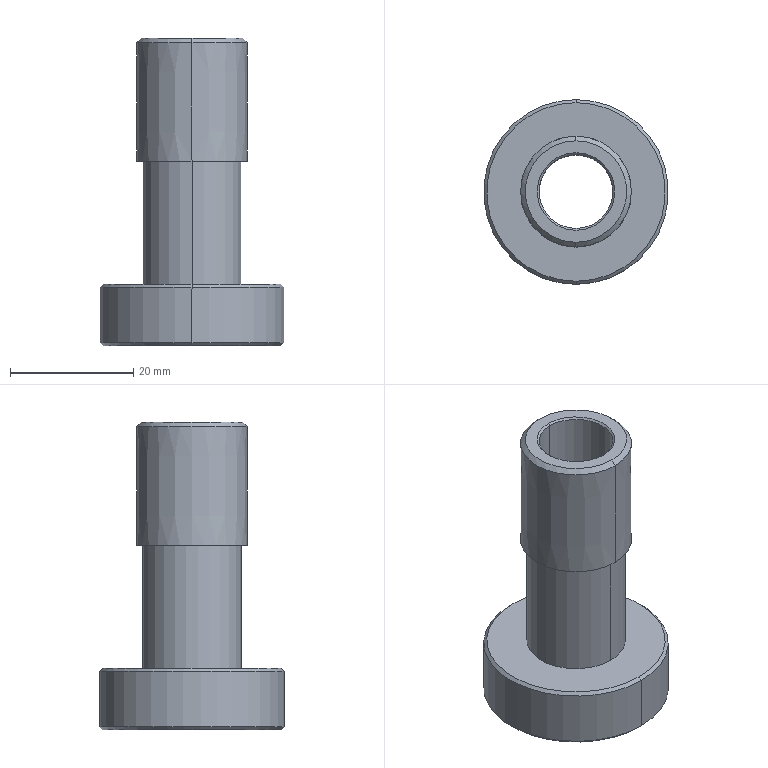Part | SolidWorks | features BaseBody 1 | 1 solid | 32 faces | box 30 x 30 x 50 mm | volume 10165 mm3 | cone 16 | cylinder 10 | plane 6 | commonest cylinder face diameters 5 x4 12 x2 16 x2 30 x2
STEP:
#1=CARTESIAN_POINT('',(590.535,44.349,-74.93));
#2=VERTEX_POINT('',#1);
#3=CARTESIAN_POINT('',(590.535,32.349,-74.93));
#4=VERTEX_POINT('',#3);
#5=CARTESIAN_POINT('',(590.535,38.349,-74.93));
#6=DIRECTION('',(0.,0.,1.));
#7=DIRECTION('',(0.,-1.,0.));
#8=AXIS2_PLACEMENT_3D('',#5,#6,#7);
#9=CIRCLE('',#8,6.);
#10=EDGE_CURVE('',#2,#4,#9,.T.);
#11=ORIENTED_EDGE('',*,*,#10,.F.);
#12=CARTESIAN_POINT('',(590.535,44.349,-25.53));
#13=VERTEX_POINT('',#12);
#14=CARTESIAN_POINT('',(590.535,44.349,-75.23));
#15=DIRECTION('',(0.,0.,1.));
#16=VECTOR('',#15,1000.);
#17=LINE('',#14,#16);
#18=EDGE_CURVE('',#2,#13,#17,.T.);
#19=ORIENTED_EDGE('',*,*,#18,.T.);
#20=CARTESIAN_POINT('',(590.535,32.349,-25.53));
#21=VERTEX_POINT('',#20);
#22=CARTESIAN_POINT('',(590.535,38.349,-25.53));
#23=DIRECTION('',(0.,0.,-1.));
#24=DIRECTION('',(0.,-1.,0.));
#25=AXIS2_PLACEMENT_3D('',#22,#23,#24);
#26=CIRCLE('',#25,6.);
#27=EDGE_CURVE('',#21,#13,#26,.T.);
#28=ORIENTED_EDGE('',*,*,#27,.F.);
#29=CARTESIAN_POINT('',(590.535,32.349,-75.23));
#30=DIRECTION('',(0.,0.,1.));
#31=VECTOR('',#30,1000.);
#32=LINE('',#29,#31);
#33=EDGE_CURVE('',#4,#21,#32,.T.);
#34=ORIENTED_EDGE('',*,*,#33,.F.);
#35=EDGE_LOOP('',(#11,#19,#28,#34));
#36=FACE_OUTER_BOUND('',#35,.T.);
#37=CARTESIAN_POINT('',(590.535,38.349,-75.23));
#38=DIRECTION('',(0.,0.,1.));
#39=DIRECTION('',(0.,-1.,0.));
#40=AXIS2_PLACEMENT_3D('',#37,#38,#39);
#41=CYLINDRICAL_SURFACE('',#40,6.);
#42=ADVANCED_FACE('',(#36),#41,.F.);
#43=ORIENTED_EDGE('',*,*,#10,.T.);
#44=CARTESIAN_POINT('',(590.535,32.049,-75.23));
#45=VERTEX_POINT('',#44);
#46=CARTESIAN_POINT('',(590.535,32.049,-75.23));
#47=DIRECTION('',(0.,-0.7071,-0.7071));
#48=VECTOR('',#47,1000.);
#49=LINE('',#46,#48);
#50=EDGE_CURVE('',#4,#45,#49,.T.);
#51=ORIENTED_EDGE('',*,*,#50,.T.);
#52=CARTESIAN_POINT('',(590.535,44.649,-75.23));
#53=VERTEX_POINT('',#52);
#54=CARTESIAN_POINT('',(590.535,38.349,-75.23));
#55=DIRECTION('',(0.,0.,1.));
#56=DIRECTION('',(0.,1.,0.));
#57=AXIS2_PLACEMENT_3D('',#54,#55,#56);
#58=CIRCLE('',#57,6.3);
#59=EDGE_CURVE('',#53,#45,#58,.T.);
#60=ORIENTED_EDGE('',*,*,#59,.F.);
#61=CARTESIAN_POINT('',(590.535,44.649,-75.23));
#62=DIRECTION('',(0.,0.7071,-0.7071));
#63=VECTOR('',#62,1000.);
#64=LINE('',#61,#63);
#65=EDGE_CURVE('',#2,#53,#64,.T.);
#66=ORIENTED_EDGE('',*,*,#65,.F.);
#67=EDGE_LOOP('',(#43,#51,#60,#66));
#68=FACE_OUTER_BOUND('',#67,.T.);
#69=CARTESIAN_POINT('',(590.535,38.349,-75.23));
#70=DIRECTION('',(0.,0.,-1.));
#71=DIRECTION('',(0.,1.,0.));
#72=AXIS2_PLACEMENT_3D('',#69,#70,#71);
#73=CONICAL_SURFACE('',#72,6.3,0.7854);
#74=ADVANCED_FACE('',(#68),#73,.F.);
#75=ORIENTED_EDGE('',*,*,#27,.T.);
#76=CARTESIAN_POINT('',(590.535,44.649,-25.23));
#77=VERTEX_POINT('',#76);
#78=CARTESIAN_POINT('',(590.535,44.649,-25.23));
#79=DIRECTION('',(0.,0.7071,0.7071));
#80=VECTOR('',#79,1000.);
#81=LINE('',#78,#80);
#82=EDGE_CURVE('',#13,#77,#81,.T.);
#83=ORIENTED_EDGE('',*,*,#82,.T.);
#84=CARTESIAN_POINT('',(590.535,32.049,-25.23));
#85=VERTEX_POINT('',#84);
#86=CARTESIAN_POINT('',(590.535,38.349,-25.23));
#87=DIRECTION('',(0.,0.,-1.));
#88=DIRECTION('',(0.,-1.,0.));
#89=AXIS2_PLACEMENT_3D('',#86,#87,#88);
#90=CIRCLE('',#89,6.3);
#91=EDGE_CURVE('',#85,#77,#90,.T.);
#92=ORIENTED_EDGE('',*,*,#91,.F.);
#93=CARTESIAN_POINT('',(590.535,32.049,-25.23));
#94=DIRECTION('',(0.,-0.7071,0.7071));
#95=VECTOR('',#94,1000.);
#96=LINE('',#93,#95);
#97=EDGE_CURVE('',#21,#85,#96,.T.);
#98=ORIENTED_EDGE('',*,*,#97,.F.);
#99=EDGE_LOOP('',(#75,#83,#92,#98));
#100=FACE_OUTER_BOUND('',#99,.T.);
#101=CARTESIAN_POINT('',(590.535,38.349,-25.23));
#102=DIRECTION('',(0.,0.,1.));
#103=DIRECTION('',(0.,-1.,0.));
#104=AXIS2_PLACEMENT_3D('',#101,#102,#103);
#105=CONICAL_SURFACE('',#104,6.3,0.7854);
#106=ADVANCED_FACE('',(#100),#105,.F.);
#107=CARTESIAN_POINT('',(596.909,43.555,-74.93));
#108=VERTEX_POINT('',#107);
#109=CARTESIAN_POINT('',(596.909,48.555,-74.93));
#110=VERTEX_POINT('',#109);
#111=CARTESIAN_POINT('',(596.909,46.055,-74.93));
#112=DIRECTION('',(0.,0.,-1.));
#113=DIRECTION('',(0.6374,0.7706,0.));
#114=AXIS2_PLACEMENT_3D('',#111,#112,#113);
#115=CIRCLE('',#114,2.5);
#116=EDGE_CURVE('',#108,#110,#115,.T.);
#117=ORIENTED_EDGE('',*,*,#116,.F.);
#118=CARTESIAN_POINT('',(596.909,43.255,-75.23));
#119=VERTEX_POINT('',#118);
#120=CARTESIAN_POINT('',(596.909,43.255,-75.23));
#121=DIRECTION('',(0.,-0.7071,-0.7071));
#122=VECTOR('',#121,1000.);
#123=LINE('',#120,#122);
#124=EDGE_CURVE('',#108,#119,#123,.T.);
#125=ORIENTED_EDGE('',*,*,#124,.T.);
#126=CARTESIAN_POINT('',(596.909,48.855,-75.23));
#127=VERTEX_POINT('',#126);
#128=CARTESIAN_POINT('',(596.909,46.055,-75.23));
#129=DIRECTION('',(0.,0.,-1.));
#130=DIRECTION('',(0.,1.,0.));
#131=AXIS2_PLACEMENT_3D('',#128,#129,#130);
#132=CIRCLE('',#131,2.8);
#133=EDGE_CURVE('',#119,#127,#132,.T.);
#134=ORIENTED_EDGE('',*,*,#133,.T.);
#135=CARTESIAN_POINT('',(596.909,48.855,-75.23));
#136=DIRECTION('',(0.,0.7071,-0.7071));
#137=VECTOR('',#136,1000.);
#138=LINE('',#135,#137);
#139=EDGE_CURVE('',#110,#127,#138,.T.);
#140=ORIENTED_EDGE('',*,*,#139,.F.);
#141=EDGE_LOOP('',(#117,#125,#134,#140));
#142=FACE_OUTER_BOUND('',#141,.T.);
#143=CARTESIAN_POINT('',(596.909,46.055,-75.23));
#144=DIRECTION('',(0.,0.,-1.));
#145=DIRECTION('',(0.,1.,0.));
#146=AXIS2_PLACEMENT_3D('',#143,#144,#145);
#147=CONICAL_SURFACE('',#146,2.8,0.7854);
#148=ADVANCED_FACE('',(#142),#147,.F.);
#149=CARTESIAN_POINT('',(590.535,23.849,-75.23));
#150=VERTEX_POINT('',#149);
#151=CARTESIAN_POINT('',(590.535,52.849,-75.23));
#152=VERTEX_POINT('',#151);
#153=CARTESIAN_POINT('',(590.535,38.349,-75.23));
#154=DIRECTION('',(0.,0.,1.));
#155=DIRECTION('',(0.,-1.,0.));
#156=AXIS2_PLACEMENT_3D('',#153,#154,#155);
#157=CIRCLE('',#156,14.5);
#158=EDGE_CURVE('',#150,#152,#157,.T.);
#159=ORIENTED_EDGE('',*,*,#158,.T.);
#160=CARTESIAN_POINT('',(590.535,53.349,-74.73));
#161=VERTEX_POINT('',#160);
#162=CARTESIAN_POINT('',(590.535,53.349,-74.73));
#163=DIRECTION('',(0.,0.7071,0.7071));
#164=VECTOR('',#163,1000.);
#165=LINE('',#162,#164);
#166=EDGE_CURVE('',#152,#161,#165,.T.);
#167=ORIENTED_EDGE('',*,*,#166,.T.);
#168=CARTESIAN_POINT('',(590.535,23.349,-74.73));
#169=VERTEX_POINT('',#168);
#170=CARTESIAN_POINT('',(590.535,38.349,-74.73));
#171=DIRECTION('',(0.,0.,-1.));
#172=DIRECTION('',(0.6374,0.7706,0.));
#173=AXIS2_PLACEMENT_3D('',#170,#171,#172);
#174=CIRCLE('',#173,15.);
#175=EDGE_CURVE('',#161,#169,#174,.T.);
#176=ORIENTED_EDGE('',*,*,#175,.T.);
#177=CARTESIAN_POINT('',(590.535,23.349,-74.73));
#178=DIRECTION('',(0.,-0.7071,0.7071));
#179=VECTOR('',#178,1000.);
#180=LINE('',#177,#179);
#181=EDGE_CURVE('',#150,#169,#180,.T.);
#182=ORIENTED_EDGE('',*,*,#181,.F.);
#183=EDGE_LOOP('',(#159,#167,#176,#182));
#184=FACE_OUTER_BOUND('',#183,.T.);
#185=CARTESIAN_POINT('',(590.535,38.349,-74.73));
#186=DIRECTION('',(0.,0.,1.));
#187=DIRECTION('',(0.,-1.,0.));
#188=AXIS2_PLACEMENT_3D('',#185,#186,#187);
#189=CONICAL_SURFACE('',#188,15.,0.7854);
#190=ADVANCED_FACE('',(#184),#189,.T.);
#191=CARTESIAN_POINT('',(584.162,28.144,-74.93));
#192=VERTEX_POINT('',#191);
#193=CARTESIAN_POINT('',(584.162,33.144,-74.93));
#194=VERTEX_POINT('',#193);
#195=CARTESIAN_POINT('',(584.162,30.644,-74.93));
#196=DIRECTION('',(0.,0.,-1.));
#197=DIRECTION('',(0.6374,0.7706,0.));
#198=AXIS2_PLACEMENT_3D('',#195,#196,#197);
#199=CIRCLE('',#198,2.5);
#200=EDGE_CURVE('',#192,#194,#199,.T.);
#201=ORIENTED_EDGE('',*,*,#200,.F.);
#202=CARTESIAN_POINT('',(584.162,27.844,-75.23));
#203=VERTEX_POINT('',#202);
#204=CARTESIAN_POINT('',(584.162,27.844,-75.23));
#205=DIRECTION('',(0.,-0.7071,-0.7071));
#206=VECTOR('',#205,1000.);
#207=LINE('',#204,#206);
#208=EDGE_CURVE('',#192,#203,#207,.T.);
#209=ORIENTED_EDGE('',*,*,#208,.T.);
#210=CARTESIAN_POINT('',(584.162,33.444,-75.23));
#211=VERTEX_POINT('',#210);
#212=CARTESIAN_POINT('',(584.162,30.644,-75.23));
#213=DIRECTION('',(0.,0.,-1.));
#214=DIRECTION('',(0.,1.,0.));
#215=AXIS2_PLACEMENT_3D('',#212,#213,#214);
#216=CIRCLE('',#215,2.8);
#217=EDGE_CURVE('',#203,#211,#216,.T.);
#218=ORIENTED_EDGE('',*,*,#217,.T.);
#219=CARTESIAN_POINT('',(584.162,33.444,-75.23));
#220=DIRECTION('',(0.,0.7071,-0.7071));
#221=VECTOR('',#220,1000.);
#222=LINE('',#219,#221);
#223=EDGE_CURVE('',#194,#211,#222,.T.);
#224=ORIENTED_EDGE('',*,*,#223,.F.);
#225=EDGE_LOOP('',(#201,#209,#218,#224));
#226=FACE_OUTER_BOUND('',#225,.T.);
#227=CARTESIAN_POINT('',(584.162,30.644,-75.23));
#228=DIRECTION('',(0.,0.,-1.));
#229=DIRECTION('',(0.,1.,0.));
#230=AXIS2_PLACEMENT_3D('',#227,#228,#229);
#231=CONICAL_SURFACE('',#230,2.8,0.7854);
#232=ADVANCED_FACE('',(#226),#231,.F.);
#233=CARTESIAN_POINT('',(590.535,30.103,-25.23));
#234=VERTEX_POINT('',#233);
#235=CARTESIAN_POINT('',(590.535,46.596,-25.23));
#236=VERTEX_POINT('',#235);
#237=CARTESIAN_POINT('',(590.535,38.349,-25.23));
#238=DIRECTION('',(0.,0.,1.));
#239=DIRECTION('',(0.,1.,0.));
#240=AXIS2_PLACEMENT_3D('',#237,#238,#239);
#241=CIRCLE('',#240,8.247);
#242=EDGE_CURVE('',#234,#236,#241,.T.);
#243=ORIENTED_EDGE('',*,*,#242,.F.);
#244=CARTESIAN_POINT('',(590.535,29.353,-25.98));
#245=VERTEX_POINT('',#244);
#246=CARTESIAN_POINT('',(590.535,29.353,-25.98));
#247=DIRECTION('',(0.,-0.7072,-0.707));
#248=VECTOR('',#247,1000.);
#249=LINE('',#246,#248);
#250=EDGE_CURVE('',#234,#245,#249,.T.);
#251=ORIENTED_EDGE('',*,*,#250,.T.);
#252=CARTESIAN_POINT('',(590.535,47.346,-25.98));
#253=VERTEX_POINT('',#252);
#254=CARTESIAN_POINT('',(590.535,38.349,-25.98));
#255=DIRECTION('',(0.,0.,1.));
#256=DIRECTION('',(0.6374,0.7706,0.));
#257=AXIS2_PLACEMENT_3D('',#254,#255,#256);
#258=CIRCLE('',#257,8.997);
#259=EDGE_CURVE('',#245,#253,#258,.T.);
#260=ORIENTED_EDGE('',*,*,#259,.T.);
#261=CARTESIAN_POINT('',(590.535,47.346,-25.98));
#262=DIRECTION('',(0.,0.7072,-0.707));
#263=VECTOR('',#262,1000.);
#264=LINE('',#261,#263);
#265=EDGE_CURVE('',#236,#253,#264,.T.);
#266=ORIENTED_EDGE('',*,*,#265,.F.);
#267=EDGE_LOOP('',(#243,#251,#260,#266));
#268=FACE_OUTER_BOUND('',#267,.T.);
#269=CARTESIAN_POINT('',(590.535,38.349,-25.98));
#270=DIRECTION('',(0.,0.,-1.));
#271=DIRECTION('',(0.,1.,0.));
#272=AXIS2_PLACEMENT_3D('',#269,#270,#271);
#273=CONICAL_SURFACE('',#272,8.997,0.7855);
#274=ADVANCED_FACE('',(#268),#273,.T.);
#275=ORIENTED_EDGE('',*,*,#116,.T.);
#276=CARTESIAN_POINT('',(596.909,48.555,-67.23));
#277=VERTEX_POINT('',#276);
#278=CARTESIAN_POINT('',(596.909,48.555,-75.23));
#279=DIRECTION('',(0.,0.,1.));
#280=VECTOR('',#279,1000.);
#281=LINE('',#278,#280);
#282=EDGE_CURVE('',#110,#277,#281,.T.);
#283=ORIENTED_EDGE('',*,*,#282,.T.);
#284=CARTESIAN_POINT('',(596.909,43.555,-67.23));
#285=VERTEX_POINT('',#284);
#286=CARTESIAN_POINT('',(596.909,46.055,-67.23));
#287=DIRECTION('',(0.,0.,-1.));
#288=DIRECTION('',(0.,-1.,0.));
#289=AXIS2_PLACEMENT_3D('',#286,#287,#288);
#290=CIRCLE('',#289,2.5);
#291=EDGE_CURVE('',#285,#277,#290,.T.);
#292=ORIENTED_EDGE('',*,*,#291,.F.);
#293=CARTESIAN_POINT('',(596.909,43.555,-75.23));
#294=DIRECTION('',(0.,0.,1.));
#295=VECTOR('',#294,1000.);
#296=LINE('',#293,#295);
#297=EDGE_CURVE('',#108,#285,#296,.T.);
#298=ORIENTED_EDGE('',*,*,#297,.F.);
#299=EDGE_LOOP('',(#275,#283,#292,#298));
#300=FACE_OUTER_BOUND('',#299,.T.);
#301=CARTESIAN_POINT('',(596.909,46.055,-75.23));
#302=DIRECTION('',(0.,0.,1.));
#303=DIRECTION('',(0.,-1.,0.));
#304=AXIS2_PLACEMENT_3D('',#301,#302,#303);
#305=CYLINDRICAL_SURFACE('',#304,2.5);
#306=ADVANCED_FACE('',(#300),#305,.F.);
#307=ORIENTED_EDGE('',*,*,#175,.F.);
#308=CARTESIAN_POINT('',(590.535,53.349,-65.73));
#309=VERTEX_POINT('',#308);
#310=CARTESIAN_POINT('',(590.535,53.349,-75.23));
#311=DIRECTION('',(0.,0.,1.));
#312=VECTOR('',#311,1000.);
#313=LINE('',#310,#312);
#314=EDGE_CURVE('',#161,#309,#313,.T.);
#315=ORIENTED_EDGE('',*,*,#314,.T.);
#316=CARTESIAN_POINT('',(590.535,23.349,-65.73));
#317=VERTEX_POINT('',#316);
#318=CARTESIAN_POINT('',(590.535,38.349,-65.73));
#319=DIRECTION('',(0.,0.,-1.));
#320=DIRECTION('',(0.,-1.,0.));
#321=AXIS2_PLACEMENT_3D('',#318,#319,#320);
#322=CIRCLE('',#321,15.);
#323=EDGE_CURVE('',#309,#317,#322,.T.);
#324=ORIENTED_EDGE('',*,*,#323,.T.);
#325=CARTESIAN_POINT('',(590.535,23.349,-75.23));
#326=DIRECTION('',(0.,0.,1.));
#327=VECTOR('',#326,1000.);
#328=LINE('',#325,#327);
#329=EDGE_CURVE('',#169,#317,#328,.T.);
#330=ORIENTED_EDGE('',*,*,#329,.F.);
#331=EDGE_LOOP('',(#307,#315,#324,#330));
#332=FACE_OUTER_BOUND('',#331,.T.);
#333=CARTESIAN_POINT('',(590.535,38.349,-75.23));
#334=DIRECTION('',(0.,0.,1.));
#335=DIRECTION('',(0.,-1.,0.));
#336=AXIS2_PLACEMENT_3D('',#333,#334,#335);
#337=CYLINDRICAL_SURFACE('',#336,15.);
#338=ADVANCED_FACE('',(#332),#337,.T.);
#339=ORIENTED_EDGE('',*,*,#200,.T.);
#340=CARTESIAN_POINT('',(584.162,33.144,-67.23));
#341=VERTEX_POINT('',#340);
#342=CARTESIAN_POINT('',(584.162,33.144,-75.23));
#343=DIRECTION('',(0.,0.,1.));
#344=VECTOR('',#343,1000.);
#345=LINE('',#342,#344);
#346=EDGE_CURVE('',#194,#341,#345,.T.);
#347=ORIENTED_EDGE('',*,*,#346,.T.);
#348=CARTESIAN_POINT('',(584.162,28.144,-67.23));
#349=VERTEX_POINT('',#348);
#350=CARTESIAN_POINT('',(584.162,30.644,-67.23));
#351=DIRECTION('',(0.,0.,-1.));
#352=DIRECTION('',(0.,-1.,0.));
#353=AXIS2_PLACEMENT_3D('',#350,#351,#352);
#354=CIRCLE('',#353,2.5);
#355=EDGE_CURVE('',#349,#341,#354,.T.);
#356=ORIENTED_EDGE('',*,*,#355,.F.);
#357=CARTESIAN_POINT('',(584.162,28.144,-75.23));
#358=DIRECTION('',(0.,0.,1.));
#359=VECTOR('',#358,1000.);
#360=LINE('',#357,#359);
#361=EDGE_CURVE('',#192,#349,#360,.T.);
#362=ORIENTED_EDGE('',*,*,#361,.F.);
#363=EDGE_LOOP('',(#339,#347,#356,#362));
#364=FACE_OUTER_BOUND('',#363,.T.);
#365=CARTESIAN_POINT('',(584.162,30.644,-75.23));
#366=DIRECTION('',(0.,0.,1.));
#367=DIRECTION('',(0.,-1.,0.));
#368=AXIS2_PLACEMENT_3D('',#365,#366,#367);
#369=CYLINDRICAL_SURFACE('',#368,2.5);
#370=ADVANCED_FACE('',(#364),#369,.F.);
#371=ORIENTED_EDGE('',*,*,#259,.F.);
#372=CARTESIAN_POINT('',(590.535,29.349,-45.23));
#373=VERTEX_POINT('',#372);
#374=CARTESIAN_POINT('',(590.535,29.349,-45.23));
#375=DIRECTION('',(0.,-0.0001745,-1.));
#376=VECTOR('',#375,1000.);
#377=LINE('',#374,#376);
#378=EDGE_CURVE('',#245,#373,#377,.T.);
#379=ORIENTED_EDGE('',*,*,#378,.T.);
#380=CARTESIAN_POINT('',(590.535,47.349,-45.23));
#381=VERTEX_POINT('',#380);
#382=CARTESIAN_POINT('',(590.535,38.349,-45.23));
#383=DIRECTION('',(0.,0.,1.));
#384=DIRECTION('',(0.,1.,0.));
#385=AXIS2_PLACEMENT_3D('',#382,#383,#384);
#386=CIRCLE('',#385,9.);
#387=EDGE_CURVE('',#373,#381,#386,.T.);
#388=ORIENTED_EDGE('',*,*,#387,.T.);
#389=CARTESIAN_POINT('',(590.535,47.349,-45.23));
#390=DIRECTION('',(0.,0.0001745,-1.));
#391=VECTOR('',#390,1000.);
#392=LINE('',#389,#391);
#393=EDGE_CURVE('',#253,#381,#392,.T.);
#394=ORIENTED_EDGE('',*,*,#393,.F.);
#395=EDGE_LOOP('',(#371,#379,#388,#394));
#396=FACE_OUTER_BOUND('',#395,.T.);
#397=CARTESIAN_POINT('',(590.535,38.349,-45.23));
#398=DIRECTION('',(0.,0.,-1.));
#399=DIRECTION('',(0.,1.,0.));
#400=AXIS2_PLACEMENT_3D('',#397,#398,#399);
#401=CONICAL_SURFACE('',#400,9.,0.0001745);
#402=ADVANCED_FACE('',(#396),#401,.T.);
#403=CARTESIAN_POINT('',(590.535,52.849,-65.23));
#404=VERTEX_POINT('',#403);
#405=CARTESIAN_POINT('',(590.535,23.849,-65.23));
#406=VERTEX_POINT('',#405);
#407=CARTESIAN_POINT('',(590.535,38.349,-65.23));
#408=DIRECTION('',(0.,0.,-1.));
#409=DIRECTION('',(0.,1.,0.));
#410=AXIS2_PLACEMENT_3D('',#407,#408,#409);
#411=CIRCLE('',#410,14.5);
#412=EDGE_CURVE('',#404,#406,#411,.T.);
#413=ORIENTED_EDGE('',*,*,#412,.T.);
#414=CARTESIAN_POINT('',(590.535,23.349,-65.73));
#415=DIRECTION('',(0.,-0.7071,-0.7071));
#416=VECTOR('',#415,1000.);
#417=LINE('',#414,#416);
#418=EDGE_CURVE('',#406,#317,#417,.T.);
#419=ORIENTED_EDGE('',*,*,#418,.T.);
#420=ORIENTED_EDGE('',*,*,#323,.F.);
#421=CARTESIAN_POINT('',(590.535,53.349,-65.73));
#422=DIRECTION('',(0.,0.7071,-0.7071));
#423=VECTOR('',#422,1000.);
#424=LINE('',#421,#423);
#425=EDGE_CURVE('',#404,#309,#424,.T.);
#426=ORIENTED_EDGE('',*,*,#425,.F.);
#427=EDGE_LOOP('',(#413,#419,#420,#426));
#428=FACE_OUTER_BOUND('',#427,.T.);
#429=CARTESIAN_POINT('',(590.535,38.349,-65.73));
#430=DIRECTION('',(0.,0.,-1.));
#431=DIRECTION('',(0.,1.,0.));
#432=AXIS2_PLACEMENT_3D('',#429,#430,#431);
#433=CONICAL_SURFACE('',#432,15.,0.7854);
#434=ADVANCED_FACE('',(#428),#433,.T.);
#435=CARTESIAN_POINT('',(590.535,46.349,-65.23));
#436=VERTEX_POINT('',#435);
#437=CARTESIAN_POINT('',(590.535,30.349,-65.23));
#438=VERTEX_POINT('',#437);
#439=CARTESIAN_POINT('',(590.535,38.349,-65.23));
#440=DIRECTION('',(0.,0.,-1.));
#441=DIRECTION('',(0.,-1.,0.));
#442=AXIS2_PLACEMENT_3D('',#439,#440,#441);
#443=CIRCLE('',#442,8.);
#444=EDGE_CURVE('',#436,#438,#443,.T.);
#445=ORIENTED_EDGE('',*,*,#444,.F.);
#446=CARTESIAN_POINT('',(590.535,46.349,-45.23));
#447=VERTEX_POINT('',#446);
#448=CARTESIAN_POINT('',(590.535,46.349,-65.23));
#449=DIRECTION('',(0.,0.,1.));
#450=VECTOR('',#449,1000.);
#451=LINE('',#448,#450);
#452=EDGE_CURVE('',#436,#447,#451,.T.);
#453=ORIENTED_EDGE('',*,*,#452,.T.);
#454=CARTESIAN_POINT('',(590.535,30.349,-45.23));
#455=VERTEX_POINT('',#454);
#456=CARTESIAN_POINT('',(590.535,38.349,-45.23));
#457=DIRECTION('',(0.,0.,-1.));
#458=DIRECTION('',(0.,-1.,0.));
#459=AXIS2_PLACEMENT_3D('',#456,#457,#458);
#460=CIRCLE('',#459,8.);
#461=EDGE_CURVE('',#447,#455,#460,.T.);
#462=ORIENTED_EDGE('',*,*,#461,.T.);
#463=CARTESIAN_POINT('',(590.535,30.349,-65.23));
#464=DIRECTION('',(0.,0.,1.));
#465=VECTOR('',#464,1000.);
#466=LINE('',#463,#465);
#467=EDGE_CURVE('',#438,#455,#466,.T.);
#468=ORIENTED_EDGE('',*,*,#467,.F.);
#469=EDGE_LOOP('',(#445,#453,#462,#468));
#470=FACE_OUTER_BOUND('',#469,.T.);
#471=CARTESIAN_POINT('',(590.535,38.349,-65.23));
#472=DIRECTION('',(0.,0.,1.));
#473=DIRECTION('',(0.,-1.,0.));
#474=AXIS2_PLACEMENT_3D('',#471,#472,#473);
#475=CYLINDRICAL_SURFACE('',#474,8.);
#476=ADVANCED_FACE('',(#470),#475,.T.);
#477=ORIENTED_EDGE('',*,*,#18,.F.);
#478=CARTESIAN_POINT('',(590.535,38.349,-74.93));
#479=DIRECTION('',(0.,0.,1.));
#480=DIRECTION('',(0.,-1.,0.));
#481=AXIS2_PLACEMENT_3D('',#478,#479,#480);
#482=CIRCLE('',#481,6.);
#483=EDGE_CURVE('',#4,#2,#482,.T.);
#484=ORIENTED_EDGE('',*,*,#483,.F.);
#485=ORIENTED_EDGE('',*,*,#33,.T.);
#486=CARTESIAN_POINT('',(590.535,38.349,-25.53));
#487=DIRECTION('',(0.,0.,-1.));
#488=DIRECTION('',(0.,-1.,0.));
#489=AXIS2_PLACEMENT_3D('',#486,#487,#488);
#490=CIRCLE('',#489,6.);
#491=EDGE_CURVE('',#13,#21,#490,.T.);
#492=ORIENTED_EDGE('',*,*,#491,.F.);
#493=EDGE_LOOP('',(#477,#484,#485,#492));
#494=FACE_OUTER_BOUND('',#493,.T.);
#495=CARTESIAN_POINT('',(590.535,38.349,-75.23));
#496=DIRECTION('',(0.,0.,1.));
#497=DIRECTION('',(0.,-1.,0.));
#498=AXIS2_PLACEMENT_3D('',#495,#496,#497);
#499=CYLINDRICAL_SURFACE('',#498,6.);
#500=ADVANCED_FACE('',(#494),#499,.F.);
#501=ORIENTED_EDGE('',*,*,#50,.F.);
#502=ORIENTED_EDGE('',*,*,#483,.T.);
#503=ORIENTED_EDGE('',*,*,#65,.T.);
#504=CARTESIAN_POINT('',(590.535,38.349,-75.23));
#505=DIRECTION('',(0.,0.,1.));
#506=DIRECTION('',(0.,1.,0.));
#507=AXIS2_PLACEMENT_3D('',#504,#505,#506);
#508=CIRCLE('',#507,6.3);
#509=EDGE_CURVE('',#45,#53,#508,.T.);
#510=ORIENTED_EDGE('',*,*,#509,.F.);
#511=EDGE_LOOP('',(#501,#502,#503,#510));
#512=FACE_OUTER_BOUND('',#511,.T.);
#513=CARTESIAN_POINT('',(590.535,38.349,-75.23));
#514=DIRECTION('',(0.,0.,-1.));
#515=DIRECTION('',(0.,1.,0.));
#516=AXIS2_PLACEMENT_3D('',#513,#514,#515);
#517=CONICAL_SURFACE('',#516,6.3,0.7854);
#518=ADVANCED_FACE('',(#512),#517,.F.);
#519=ORIENTED_EDGE('',*,*,#82,.F.);
#520=ORIENTED_EDGE('',*,*,#491,.T.);
#521=ORIENTED_EDGE('',*,*,#97,.T.);
#522=CARTESIAN_POINT('',(590.535,38.349,-25.23));
#523=DIRECTION('',(0.,0.,-1.));
#524=DIRECTION('',(0.,-1.,0.));
#525=AXIS2_PLACEMENT_3D('',#522,#523,#524);
#526=CIRCLE('',#525,6.3);
#527=EDGE_CURVE('',#77,#85,#526,.T.);
#528=ORIENTED_EDGE('',*,*,#527,.F.);
#529=EDGE_LOOP('',(#519,#520,#521,#528));
#530=FACE_OUTER_BOUND('',#529,.T.);
#531=CARTESIAN_POINT('',(590.535,38.349,-25.23));
#532=DIRECTION('',(0.,0.,1.));
#533=DIRECTION('',(0.,-1.,0.));
#534=AXIS2_PLACEMENT_3D('',#531,#532,#533);
#535=CONICAL_SURFACE('',#534,6.3,0.7854);
#536=ADVANCED_FACE('',(#530),#535,.F.);
#537=ORIENTED_EDGE('',*,*,#59,.T.);
#538=ORIENTED_EDGE('',*,*,#509,.T.);
#539=EDGE_LOOP('',(#537,#538));
#540=FACE_BOUND('',#539,.T.);
#541=CARTESIAN_POINT('',(596.909,46.055,-75.23));
#542=DIRECTION('',(0.,0.,-1.));
#543=DIRECTION('',(0.,1.,0.));
#544=AXIS2_PLACEMENT_3D('',#541,#542,#543);
#545=CIRCLE('',#544,2.8);
#546=EDGE_CURVE('',#127,#119,#545,.T.);
#547=ORIENTED_EDGE('',*,*,#546,.F.);
#548=ORIENTED_EDGE('',*,*,#133,.F.);
#549=EDGE_LOOP('',(#547,#548));
#550=FACE_BOUND('',#549,.T.);
#551=ORIENTED_EDGE('',*,*,#158,.F.);
#552=CARTESIAN_POINT('',(590.535,38.349,-75.23));
#553=DIRECTION('',(0.,0.,1.));
#554=DIRECTION('',(0.,-1.,0.));
#555=AXIS2_PLACEMENT_3D('',#552,#553,#554);
#556=CIRCLE('',#555,14.5);
#557=EDGE_CURVE('',#152,#150,#556,.T.);
#558=ORIENTED_EDGE('',*,*,#557,.F.);
#559=EDGE_LOOP('',(#551,#558));
#560=FACE_OUTER_BOUND('',#559,.T.);
#561=CARTESIAN_POINT('',(584.162,30.644,-75.23));
#562=DIRECTION('',(0.,0.,-1.));
#563=DIRECTION('',(0.,1.,0.));
#564=AXIS2_PLACEMENT_3D('',#561,#562,#563);
#565=CIRCLE('',#564,2.8);
#566=EDGE_CURVE('',#211,#203,#565,.T.);
#567=ORIENTED_EDGE('',*,*,#566,.F.);
#568=ORIENTED_EDGE('',*,*,#217,.F.);
#569=EDGE_LOOP('',(#567,#568));
#570=FACE_BOUND('',#569,.T.);
#571=CARTESIAN_POINT('',(590.535,38.349,-75.23));
#572=DIRECTION('',(0.,0.,1.));
#573=DIRECTION('',(0.,-1.,0.));
#574=AXIS2_PLACEMENT_3D('',#571,#572,#573);
#575=PLANE('',#574);
#576=ADVANCED_FACE('',(#540,#550,#560,#570),#575,.F.);
#577=ORIENTED_EDGE('',*,*,#91,.T.);
#578=ORIENTED_EDGE('',*,*,#527,.T.);
#579=EDGE_LOOP('',(#577,#578));
#580=FACE_BOUND('',#579,.T.);
#581=CARTESIAN_POINT('',(590.535,38.349,-25.23));
#582=DIRECTION('',(0.,0.,1.));
#583=DIRECTION('',(0.,1.,0.));
#584=AXIS2_PLACEMENT_3D('',#581,#582,#583);
#585=CIRCLE('',#584,8.247);
#586=EDGE_CURVE('',#236,#234,#585,.T.);
#587=ORIENTED_EDGE('',*,*,#586,.T.);
#588=ORIENTED_EDGE('',*,*,#242,.T.);
#589=EDGE_LOOP('',(#587,#588));
#590=FACE_OUTER_BOUND('',#589,.T.);
#591=CARTESIAN_POINT('',(590.535,38.349,-25.23));
#592=DIRECTION('',(0.,0.,1.));
#593=DIRECTION('',(0.,-1.,0.));
#594=AXIS2_PLACEMENT_3D('',#591,#592,#593);
#595=PLANE('',#594);
#596=ADVANCED_FACE('',(#580,#590),#595,.T.);
#597=ORIENTED_EDGE('',*,*,#124,.F.);
#598=CARTESIAN_POINT('',(596.909,46.055,-74.93));
#599=DIRECTION('',(0.,0.,-1.));
#600=DIRECTION('',(0.6374,0.7706,0.));
#601=AXIS2_PLACEMENT_3D('',#598,#599,#600);
#602=CIRCLE('',#601,2.5);
#603=EDGE_CURVE('',#110,#108,#602,.T.);
#604=ORIENTED_EDGE('',*,*,#603,.F.);
#605=ORIENTED_EDGE('',*,*,#139,.T.);
#606=ORIENTED_EDGE('',*,*,#546,.T.);
#607=EDGE_LOOP('',(#597,#604,#605,#606));
#608=FACE_OUTER_BOUND('',#607,.T.);
#609=CARTESIAN_POINT('',(596.909,46.055,-75.23));
#610=DIRECTION('',(0.,0.,-1.));
#611=DIRECTION('',(0.,1.,0.));
#612=AXIS2_PLACEMENT_3D('',#609,#610,#611);
#613=CONICAL_SURFACE('',#612,2.8,0.7854);
#614=ADVANCED_FACE('',(#608),#613,.F.);
#615=ORIENTED_EDGE('',*,*,#166,.F.);
#616=ORIENTED_EDGE('',*,*,#557,.T.);
#617=ORIENTED_EDGE('',*,*,#181,.T.);
#618=CARTESIAN_POINT('',(590.535,38.349,-74.73));
#619=DIRECTION('',(0.,0.,-1.));
#620=DIRECTION('',(0.6374,0.7706,0.));
#621=AXIS2_PLACEMENT_3D('',#618,#619,#620);
#622=CIRCLE('',#621,15.);
#623=EDGE_CURVE('',#169,#161,#622,.T.);
#624=ORIENTED_EDGE('',*,*,#623,.T.);
#625=EDGE_LOOP('',(#615,#616,#617,#624));
#626=FACE_OUTER_BOUND('',#625,.T.);
#627=CARTESIAN_POINT('',(590.535,38.349,-74.73));
#628=DIRECTION('',(0.,0.,1.));
#629=DIRECTION('',(0.,-1.,0.));
#630=AXIS2_PLACEMENT_3D('',#627,#628,#629);
#631=CONICAL_SURFACE('',#630,15.,0.7854);
#632=ADVANCED_FACE('',(#626),#631,.T.);
#633=ORIENTED_EDGE('',*,*,#208,.F.);
#634=CARTESIAN_POINT('',(584.162,30.644,-74.93));
#635=DIRECTION('',(0.,0.,-1.));
#636=DIRECTION('',(0.6374,0.7706,0.));
#637=AXIS2_PLACEMENT_3D('',#634,#635,#636);
#638=CIRCLE('',#637,2.5);
#639=EDGE_CURVE('',#194,#192,#638,.T.);
#640=ORIENTED_EDGE('',*,*,#639,.F.);
#641=ORIENTED_EDGE('',*,*,#223,.T.);
#642=ORIENTED_EDGE('',*,*,#566,.T.);
#643=EDGE_LOOP('',(#633,#640,#641,#642));
#644=FACE_OUTER_BOUND('',#643,.T.);
#645=CARTESIAN_POINT('',(584.162,30.644,-75.23));
#646=DIRECTION('',(0.,0.,-1.));
#647=DIRECTION('',(0.,1.,0.));
#648=AXIS2_PLACEMENT_3D('',#645,#646,#647);
#649=CONICAL_SURFACE('',#648,2.8,0.7854);
#650=ADVANCED_FACE('',(#644),#649,.F.);
#651=ORIENTED_EDGE('',*,*,#250,.F.);
#652=ORIENTED_EDGE('',*,*,#586,.F.);
#653=ORIENTED_EDGE('',*,*,#265,.T.);
#654=CARTESIAN_POINT('',(590.535,38.349,-25.98));
#655=DIRECTION('',(0.,0.,1.));
#656=DIRECTION('',(0.6374,0.7706,0.));
#657=AXIS2_PLACEMENT_3D('',#654,#655,#656);
#658=CIRCLE('',#657,8.997);
#659=EDGE_CURVE('',#253,#245,#658,.T.);
#660=ORIENTED_EDGE('',*,*,#659,.T.);
#661=EDGE_LOOP('',(#651,#652,#653,#660));
#662=FACE_OUTER_BOUND('',#661,.T.);
#663=CARTESIAN_POINT('',(590.535,38.349,-25.98));
#664=DIRECTION('',(0.,0.,-1.));
#665=DIRECTION('',(0.,1.,0.));
#666=AXIS2_PLACEMENT_3D('',#663,#664,#665);
#667=CONICAL_SURFACE('',#666,8.997,0.7855);
#668=ADVANCED_FACE('',(#662),#667,.T.);
#669=ORIENTED_EDGE('',*,*,#282,.F.);
#670=ORIENTED_EDGE('',*,*,#603,.T.);
#671=ORIENTED_EDGE('',*,*,#297,.T.);
#672=CARTESIAN_POINT('',(596.909,46.055,-67.23));
#673=DIRECTION('',(0.,0.,-1.));
#674=DIRECTION('',(0.,-1.,0.));
#675=AXIS2_PLACEMENT_3D('',#672,#673,#674);
#676=CIRCLE('',#675,2.5);
#677=EDGE_CURVE('',#277,#285,#676,.T.);
#678=ORIENTED_EDGE('',*,*,#677,.F.);
#679=EDGE_LOOP('',(#669,#670,#671,#678));
#680=FACE_OUTER_BOUND('',#679,.T.);
#681=CARTESIAN_POINT('',(596.909,46.055,-75.23));
#682=DIRECTION('',(0.,0.,1.));
#683=DIRECTION('',(0.,-1.,0.));
#684=AXIS2_PLACEMENT_3D('',#681,#682,#683);
#685=CYLINDRICAL_SURFACE('',#684,2.5);
#686=ADVANCED_FACE('',(#680),#685,.F.);
#687=ORIENTED_EDGE('',*,*,#314,.F.);
#688=ORIENTED_EDGE('',*,*,#623,.F.);
#689=ORIENTED_EDGE('',*,*,#329,.T.);
#690=CARTESIAN_POINT('',(590.535,38.349,-65.73));
#691=DIRECTION('',(0.,0.,-1.));
#692=DIRECTION('',(0.,-1.,0.));
#693=AXIS2_PLACEMENT_3D('',#690,#691,#692);
#694=CIRCLE('',#693,15.);
#695=EDGE_CURVE('',#317,#309,#694,.T.);
#696=ORIENTED_EDGE('',*,*,#695,.T.);
#697=EDGE_LOOP('',(#687,#688,#689,#696));
#698=FACE_OUTER_BOUND('',#697,.T.);
#699=CARTESIAN_POINT('',(590.535,38.349,-75.23));
#700=DIRECTION('',(0.,0.,1.));
#701=DIRECTION('',(0.,-1.,0.));
#702=AXIS2_PLACEMENT_3D('',#699,#700,#701);
#703=CYLINDRICAL_SURFACE('',#702,15.);
#704=ADVANCED_FACE('',(#698),#703,.T.);
#705=ORIENTED_EDGE('',*,*,#346,.F.);
#706=ORIENTED_EDGE('',*,*,#639,.T.);
#707=ORIENTED_EDGE('',*,*,#361,.T.);
#708=CARTESIAN_POINT('',(584.162,30.644,-67.23));
#709=DIRECTION('',(0.,0.,-1.));
#710=DIRECTION('',(0.,-1.,0.));
#711=AXIS2_PLACEMENT_3D('',#708,#709,#710);
#712=CIRCLE('',#711,2.5);
#713=EDGE_CURVE('',#341,#349,#712,.T.);
#714=ORIENTED_EDGE('',*,*,#713,.F.);
#715=EDGE_LOOP('',(#705,#706,#707,#714));
#716=FACE_OUTER_BOUND('',#715,.T.);
#717=CARTESIAN_POINT('',(584.162,30.644,-75.23));
#718=DIRECTION('',(0.,0.,1.));
#719=DIRECTION('',(0.,-1.,0.));
#720=AXIS2_PLACEMENT_3D('',#717,#718,#719);
#721=CYLINDRICAL_SURFACE('',#720,2.5);
#722=ADVANCED_FACE('',(#716),#721,.F.);
#723=ORIENTED_EDGE('',*,*,#378,.F.);
#724=ORIENTED_EDGE('',*,*,#659,.F.);
#725=ORIENTED_EDGE('',*,*,#393,.T.);
#726=CARTESIAN_POINT('',(590.535,38.349,-45.23));
#727=DIRECTION('',(0.,0.,1.));
#728=DIRECTION('',(0.,1.,0.));
#729=AXIS2_PLACEMENT_3D('',#726,#727,#728);
#730=CIRCLE('',#729,9.);
#731=EDGE_CURVE('',#381,#373,#730,.T.);
#732=ORIENTED_EDGE('',*,*,#731,.T.);
#733=EDGE_LOOP('',(#723,#724,#725,#732));
#734=FACE_OUTER_BOUND('',#733,.T.);
#735=CARTESIAN_POINT('',(590.535,38.349,-45.23));
#736=DIRECTION('',(0.,0.,-1.));
#737=DIRECTION('',(0.,1.,0.));
#738=AXIS2_PLACEMENT_3D('',#735,#736,#737);
#739=CONICAL_SURFACE('',#738,9.,0.0001745);
#740=ADVANCED_FACE('',(#734),#739,.T.);
#741=ORIENTED_EDGE('',*,*,#291,.T.);
#742=ORIENTED_EDGE('',*,*,#677,.T.);
#743=EDGE_LOOP('',(#741,#742));
#744=FACE_OUTER_BOUND('',#743,.T.);
#745=CARTESIAN_POINT('',(596.909,46.055,-67.23));
#746=DIRECTION('',(0.,0.,1.));
#747=DIRECTION('',(0.,-1.,0.));
#748=AXIS2_PLACEMENT_3D('',#745,#746,#747);
#749=PLANE('',#748);
#750=ADVANCED_FACE('',(#744),#749,.F.);
#751=ORIENTED_EDGE('',*,*,#418,.F.);
#752=CARTESIAN_POINT('',(590.535,38.349,-65.23));
#753=DIRECTION('',(0.,0.,-1.));
#754=DIRECTION('',(0.,1.,0.));
#755=AXIS2_PLACEMENT_3D('',#752,#753,#754);
#756=CIRCLE('',#755,14.5);
#757=EDGE_CURVE('',#406,#404,#756,.T.);
#758=ORIENTED_EDGE('',*,*,#757,.T.);
#759=ORIENTED_EDGE('',*,*,#425,.T.);
#760=ORIENTED_EDGE('',*,*,#695,.F.);
#761=EDGE_LOOP('',(#751,#758,#759,#760));
#762=FACE_OUTER_BOUND('',#761,.T.);
#763=CARTESIAN_POINT('',(590.535,38.349,-65.73));
#764=DIRECTION('',(0.,0.,-1.));
#765=DIRECTION('',(0.,1.,0.));
#766=AXIS2_PLACEMENT_3D('',#763,#764,#765);
#767=CONICAL_SURFACE('',#766,15.,0.7854);
#768=ADVANCED_FACE('',(#762),#767,.T.);
#769=ORIENTED_EDGE('',*,*,#355,.T.);
#770=ORIENTED_EDGE('',*,*,#713,.T.);
#771=EDGE_LOOP('',(#769,#770));
#772=FACE_OUTER_BOUND('',#771,.T.);
#773=CARTESIAN_POINT('',(584.162,30.644,-67.23));
#774=DIRECTION('',(0.,0.,1.));
#775=DIRECTION('',(0.,-1.,0.));
#776=AXIS2_PLACEMENT_3D('',#773,#774,#775);
#777=PLANE('',#776);
#778=ADVANCED_FACE('',(#772),#777,.F.);
#779=ORIENTED_EDGE('',*,*,#731,.F.);
#780=ORIENTED_EDGE('',*,*,#387,.F.);
#781=EDGE_LOOP('',(#779,#780));
#782=FACE_OUTER_BOUND('',#781,.T.);
#783=CARTESIAN_POINT('',(590.535,38.349,-45.23));
#784=DIRECTION('',(0.,0.,-1.));
#785=DIRECTION('',(0.,-1.,0.));
#786=AXIS2_PLACEMENT_3D('',#783,#784,#785);
#787=CIRCLE('',#786,8.);
#788=EDGE_CURVE('',#455,#447,#787,.T.);
#789=ORIENTED_EDGE('',*,*,#788,.F.);
#790=ORIENTED_EDGE('',*,*,#461,.F.);
#791=EDGE_LOOP('',(#789,#790));
#792=FACE_BOUND('',#791,.T.);
#793=CARTESIAN_POINT('',(590.535,38.349,-45.23));
#794=DIRECTION('',(0.,0.,1.));
#795=DIRECTION('',(0.,-1.,0.));
#796=AXIS2_PLACEMENT_3D('',#793,#794,#795);
#797=PLANE('',#796);
#798=ADVANCED_FACE('',(#782,#792),#797,.F.);
#799=ORIENTED_EDGE('',*,*,#412,.F.);
#800=ORIENTED_EDGE('',*,*,#757,.F.);
#801=EDGE_LOOP('',(#799,#800));
#802=FACE_OUTER_BOUND('',#801,.T.);
#803=CARTESIAN_POINT('',(590.535,38.349,-65.23));
#804=DIRECTION('',(0.,0.,-1.));
#805=DIRECTION('',(0.,-1.,0.));
#806=AXIS2_PLACEMENT_3D('',#803,#804,#805);
#807=CIRCLE('',#806,8.);
#808=EDGE_CURVE('',#438,#436,#807,.T.);
#809=ORIENTED_EDGE('',*,*,#808,.T.);
#810=ORIENTED_EDGE('',*,*,#444,.T.);
#811=EDGE_LOOP('',(#809,#810));
#812=FACE_BOUND('',#811,.T.);
#813=CARTESIAN_POINT('',(590.535,38.349,-65.23));
#814=DIRECTION('',(0.,0.,1.));
#815=DIRECTION('',(0.,-1.,0.));
#816=AXIS2_PLACEMENT_3D('',#813,#814,#815);
#817=PLANE('',#816);
#818=ADVANCED_FACE('',(#802,#812),#817,.T.);
#819=ORIENTED_EDGE('',*,*,#452,.F.);
#820=ORIENTED_EDGE('',*,*,#808,.F.);
#821=ORIENTED_EDGE('',*,*,#467,.T.);
#822=ORIENTED_EDGE('',*,*,#788,.T.);
#823=EDGE_LOOP('',(#819,#820,#821,#822));
#824=FACE_OUTER_BOUND('',#823,.T.);
#825=CARTESIAN_POINT('',(590.535,38.349,-65.23));
#826=DIRECTION('',(0.,0.,1.));
#827=DIRECTION('',(0.,-1.,0.));
#828=AXIS2_PLACEMENT_3D('',#825,#826,#827);
#829=CYLINDRICAL_SURFACE('',#828,8.);
#830=ADVANCED_FACE('',(#824),#829,.T.);
#831=CLOSED_SHELL('',(#42,#74,#106,#148,#190,#232,#274,#306,#338,#370,#402,#434,#476,#500,#518,#536,#576,#596,#614,#632,#650,#668,#686,#704,#722,#740,#750,#768,#778,#798,#818,#830));
#832=MANIFOLD_SOLID_BREP('',#831);
#833=CARTESIAN_POINT('',(0.,0.,0.));
#834=DIRECTION('',(0.,0.,1.));
#835=DIRECTION('',(1.,0.,0.));
#836=AXIS2_PLACEMENT_3D('',#833,#834,#835);
#837=(LENGTH_UNIT()NAMED_UNIT(*)SI_UNIT(.MILLI.,.METRE.));
#838=UNCERTAINTY_MEASURE_WITH_UNIT(LENGTH_MEASURE(0.00001),#837,'','');
#839=(NAMED_UNIT(*)PLANE_ANGLE_UNIT()SI_UNIT($,.RADIAN.));
#840=(NAMED_UNIT(*)SI_UNIT($,.STERADIAN.)SOLID_ANGLE_UNIT());
#841=(GEOMETRIC_REPRESENTATION_CONTEXT(3)GLOBAL_UNCERTAINTY_ASSIGNED_CONTEXT((#838))GLOBAL_UNIT_ASSIGNED_CONTEXT((#837,#839,#840))REPRESENTATION_CONTEXT('',''));
#842=ADVANCED_BREP_SHAPE_REPRESENTATION('',(#832,#836),#841);